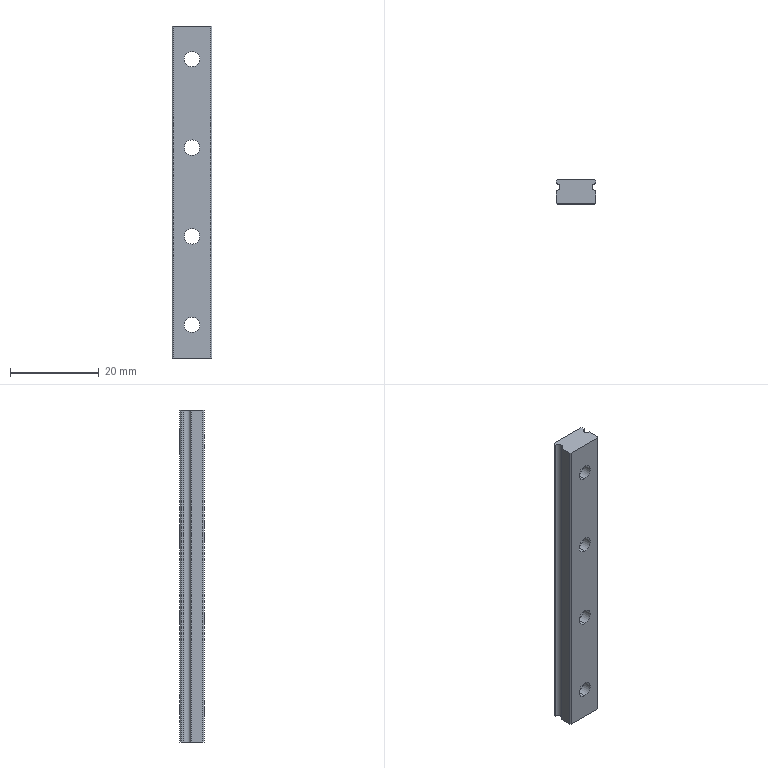Part | STEP file | Linear rail | 1 solid | 35 faces | box 9 x 5.5 x 75 mm | volume 3056 mm3 | cylinder 19 | plane 16 | commonest cylinder face diameters 3.5 x8 6 x8 1.7 x3